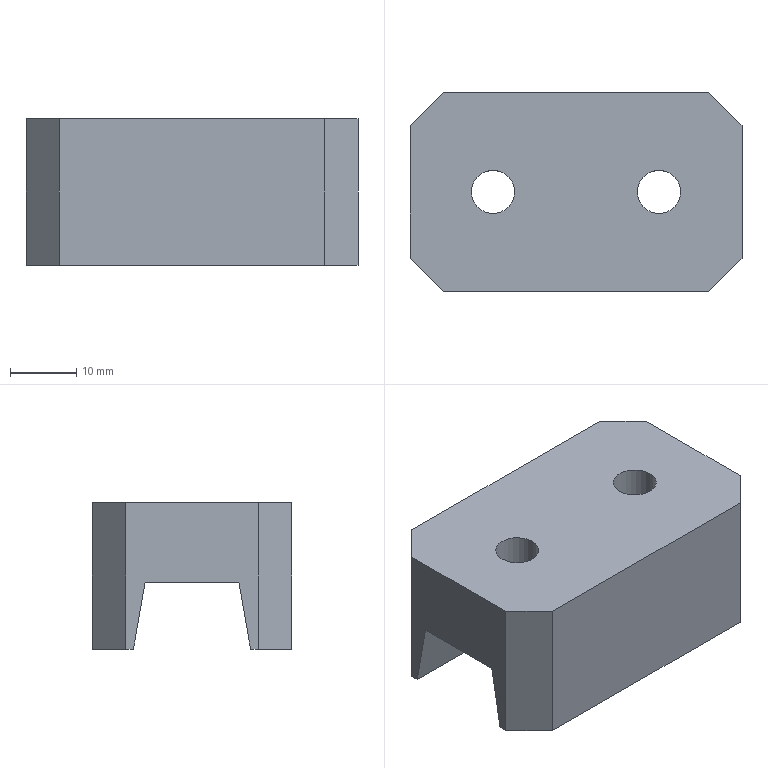Part | STEP file | solid 102 | 1 solid | 20 faces | box 50 x 30 x 22 mm | volume 22296 mm3 | plane 16 | cylinder 4 | commonest cylinder face diameters 6.5 x2 11 x2